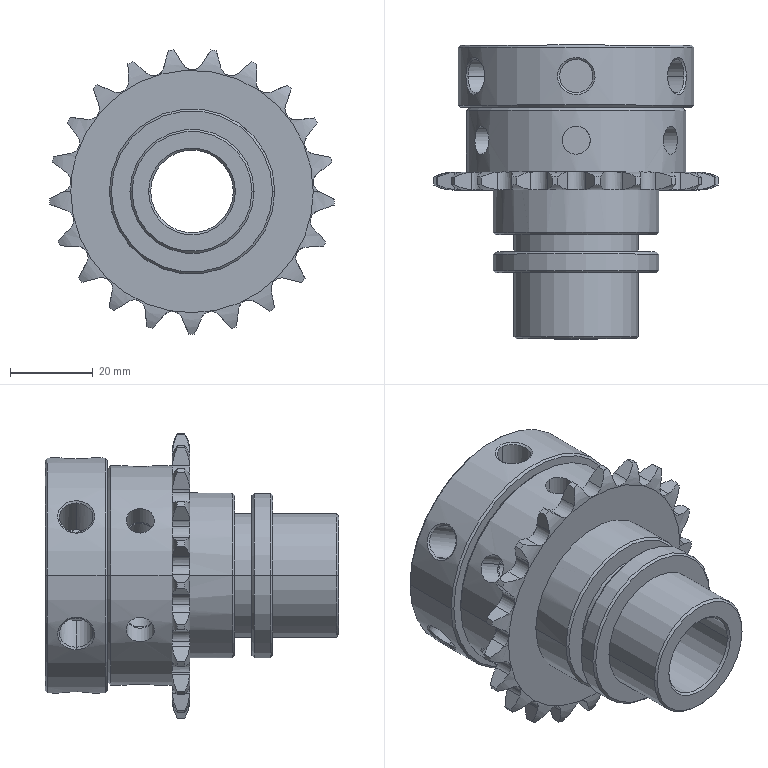Part | SolidWorks | 2 solids | 210 faces | box 69 x 71 x 68.718 mm | volume 90688 mm3 | cylinder 101 | plane 63 | spline 28 | cone 18 | commonest cylinder face diameters 5.2 x28 6.8 x24 69 x21 8.1 x12 40 x6 30 x4